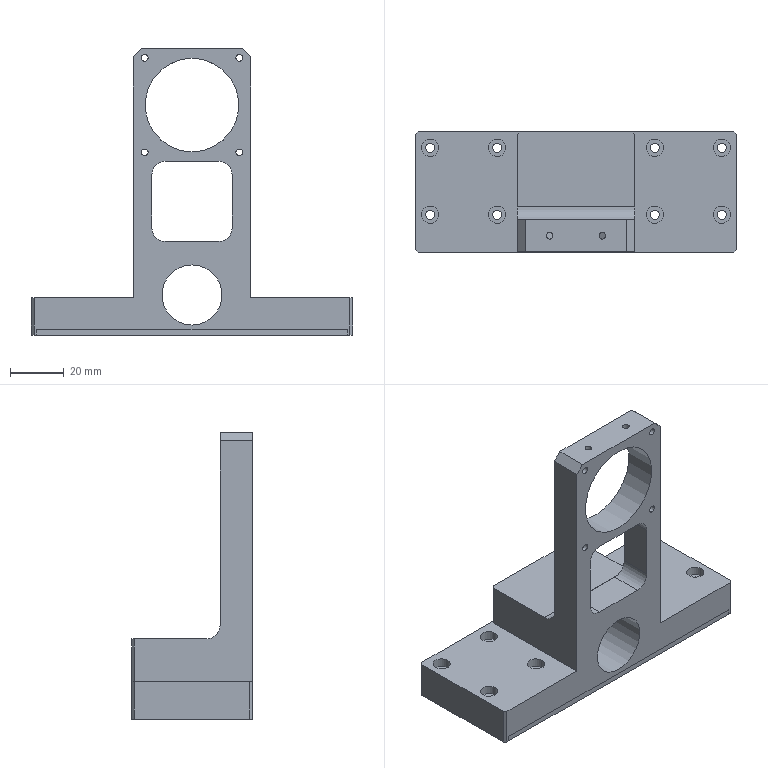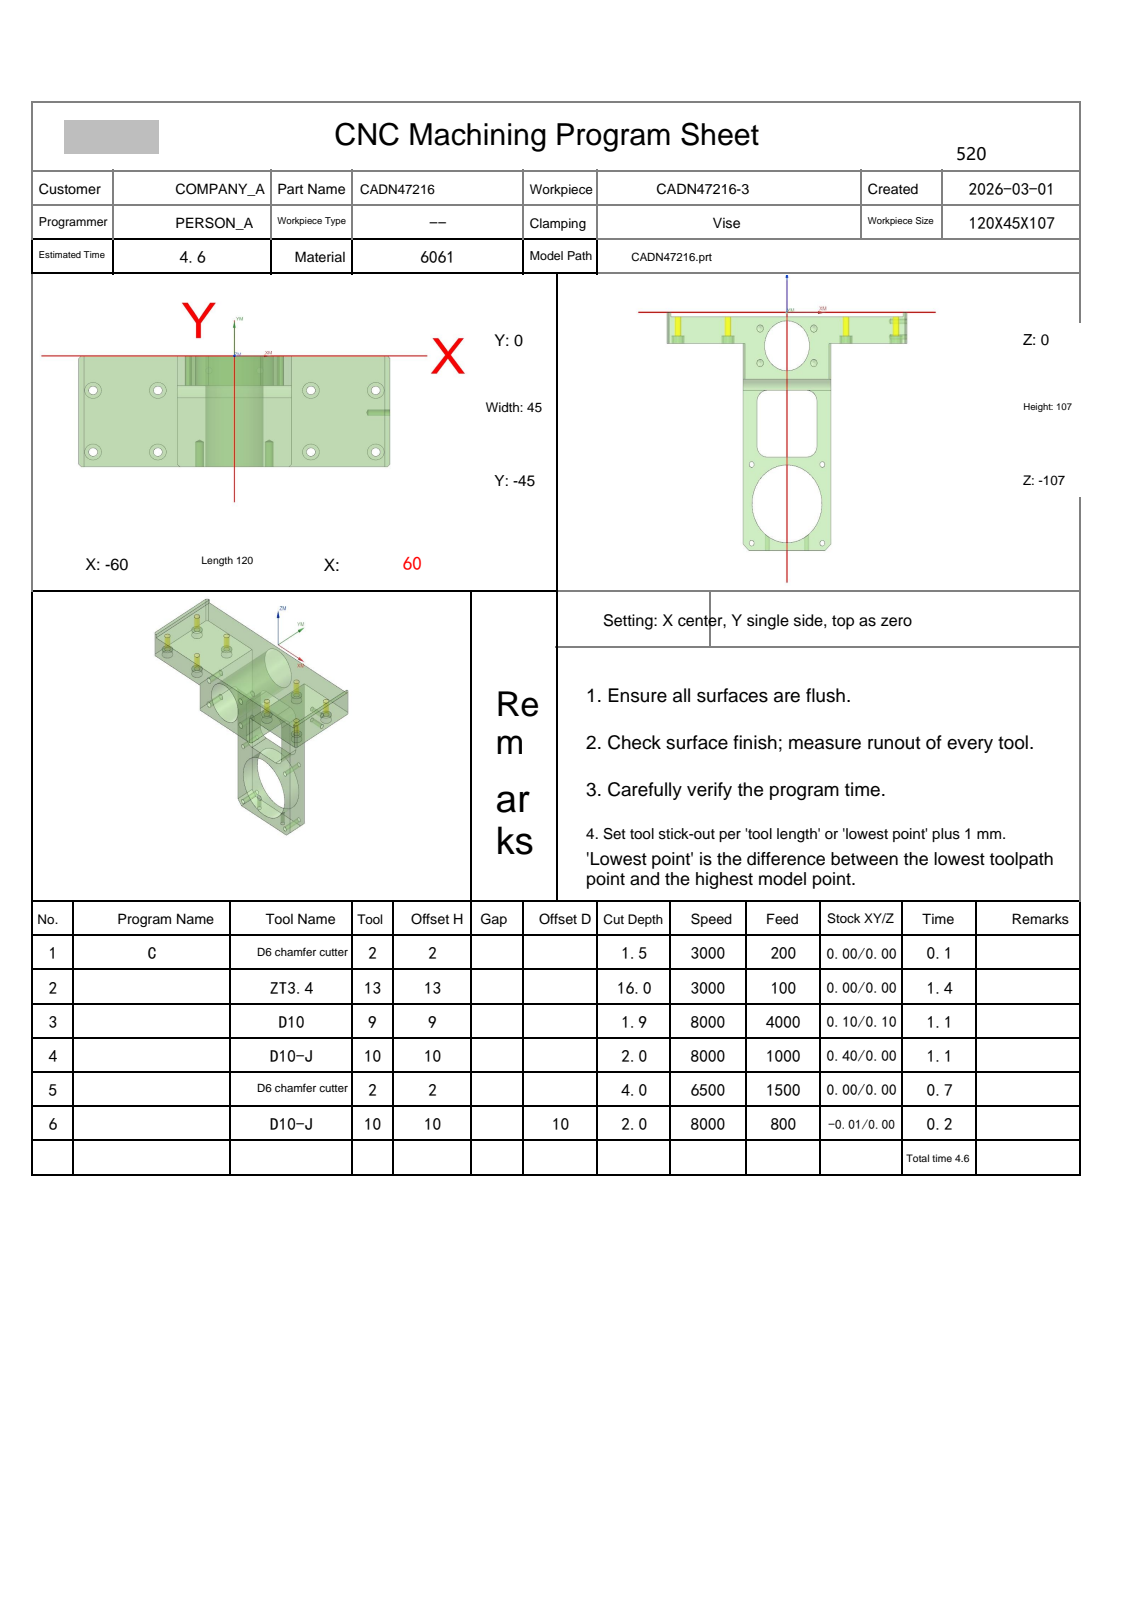NC program | NX | posted by the shop | part box 120 x 45 x 107 mm
Whole program:
%
O0001
(Machine time: 5.76 MIN)
(===Total Tool:4===)
(T2=D6 chamfer cutter   D=6.   R=0.   D-  H02 Z=-4.   )
(T13=ZT3.4  D=3.4  DR_a=118 D-  H13 Z=-16.  )
(T9=D10     D=10.  R=0.   D-  H09 Z=-1.9  )
(T10=D10-J  D=10.  R=0.   D-  H10 Z=-2.   )
G80 G90 G17 G49 G40
G91 G28 Z0
M01
N1 T02 M06
(D6 chamfer cutter  D=6. R=0. H=02 ce=0.00 di=0.00)
G00 G90 G54 X-29.5 Y-14. M03 S3000
G43 H02 Z50.
M08
G98 G81 X-29.5 Y-14. Z-1.5 R1. F200.
X-54.5
Y-39.
X-29.5
X29.5
X54.5
Y-14.
X29.5
G80
G00 Z50.
G91 G28 Z0.0
M05
M09
G91 G28 Z0.0
M01
N2 T13 M06
(ZT3.4 D=3.4 DR_a=118 H=13)
G00 G90 G54 X-29.5 Y-14. M03 S3000
G43 H13 Z50.
M08
G98 G83 X-29.5 Y-14. Z-16. R1. F100. Q1.5
X-54.5
Y-39.
X-29.5
X29.5
X54.5
Y-14.
X29.5
G80
G00 Z50.
G91 G28 Z0.0
M05
M09
G91 G28 Z0.0
M01
N3 T09 M06
(D10  D=10. R=0. H=09 ce=0.10 di=0.10)
G00 G90 G54 X0.0 Y-53. M03 S8000
G43 H09 Z10.1
M08
Z1.025
G01 Z-.475 F4000.
Y-49.9
X-52.9
Y4.9
X52.9
Y-49.9
X3.035
G02 X2.203 Y-49.455 I.001 J1.
G01 X-2.203 Y-42.845
G03 X-3.035 Y-42.4 I-.832 J-.555
G01 X-44.403
G02 X-45.4 Y-41.403 I.003 J1.
G01 Y-3.597
G02 X-44.403 Y-2.6 I1. J-.003
G01 X44.403
G02 X45.4 Y-3.597 I-.003 J-1.
G01 Y-41.403
G02 X44.403 Y-42.4 I-1. J.003
G01 X3.035
G02 X2.203 Y-41.955 I.001 J1.
G01 X-2.203 Y-35.345
G03 X-3.035 Y-34.9 I-.832 J-.555
G01 X-36.903
G02 X-37.9 Y-33.903 I.003 J1.
G01 Y-11.097
G02 X-36.903 Y-10.1 I1. J-.003
G01 X36.903
G02 X37.9 Y-11.097 I-.003 J-1.
G01 Y-33.903
G02 X36.903 Y-34.9 I-1. J.003
G01 X3.035
G02 X2.203 Y-34.455 I0.0 J1.
G01 X-2.203 Y-27.845
G03 X-3.035 Y-27.4 I-.832 J-.555
G01 X-29.403
G02 X-30.4 Y-26.403 I.003 J1.
G01 Y-18.597
G02 X-29.403 Y-17.6 I1. J-.003
G01 X29.403
G02 X30.4 Y-18.597 I-.003 J-1.
G01 Y-26.403
G02 X29.403 Y-27.4 I-1. J.003
G01 X2.664
G02 X1.957 Y-27.107 I0.0 J1.
G01 X-1.957 Y-23.193
G03 X-2.664 Y-22.9 I-.707 J-.707
G01 X-25.502
G02 X-25.9 Y-22.5 I.002 J.4
X-25.502 Y-22.1 I.4 J0.0
G01 X25.502
G02 X25.9 Y-22.5 I-.002 J-.4
X25.502 Y-22.9 I-.4 J0.0
G01 X0.0
X-.5
Y-25.9
Z1.025
G00 X0.0 Y-53.
Z.55
G01 Z-.95
Y-49.9
X-52.9
Y4.9
X52.9
Y-49.9
X3.035
G02 X2.203 Y-49.455 I.001 J1.
G01 X-2.203 Y-42.845
G03 X-3.035 Y-42.4 I-.832 J-.555
G01 X-44.403
G02 X-45.4 Y-41.403 I.003 J1.
G01 Y-3.597
G02 X-44.403 Y-2.6 I1. J-.003
G01 X44.403
G02 X45.4 Y-3.597 I-.003 J-1.
G01 Y-41.403
G02 X44.403 Y-42.4 I-1. J.003
G01 X3.035
G02 X2.203 Y-41.955 I.001 J1.
G01 X-2.203 Y-35.345
G03 X-3.035 Y-34.9 I-.832 J-.555
G01 X-36.903
G02 X-37.9 Y-33.903 I.003 J1.
G01 Y-11.097
G02 X-36.903 Y-10.1 I1. J-.003
G01 X36.903
G02 X37.9 Y-11.097 I-.003 J-1.
G01 Y-33.903
G02 X36.903 Y-34.9 I-1. J.003
G01 X3.035
G02 X2.203 Y-34.455 I0.0 J1.
G01 X-2.203 Y-27.845
G03 X-3.035 Y-27.4 I-.832 J-.555
G01 X-29.403
G02 X-30.4 Y-26.403 I.003 J1.
G01 Y-18.597
G02 X-29.403 Y-17.6 I1. J-.003
G01 X29.403
G02 X30.4 Y-18.597 I-.003 J-1.
G01 Y-26.403
G02 X29.403 Y-27.4 I-1. J.003
G01 X2.664
G02 X1.957 Y-27.107 I0.0 J1.
G01 X-1.957 Y-23.193
G03 X-2.664 Y-22.9 I-.707 J-.707
G01 X-25.502
G02 X-25.9 Y-22.5 I.002 J.4
X-25.502 Y-22.1 I.4 J0.0
G01 X25.502
G02 X25.9 Y-22.5 I-.002 J-.4
X25.502 Y-22.9 I-.4 J0.0
G01 X0.0
X-.5
Y-25.9
Z.55
G00 X0.0 Y-53.
Z.075
G01 Z-1.425
Y-49.9
X-52.9
Y4.9
X52.9
Y-49.9
X3.035
G02 X2.203 Y-49.455 I.001 J1.
G01 X-2.203 Y-42.845
G03 X-3.035 Y-42.4 I-.832 J-.555
G01 X-44.403
G02 X-45.4 Y-41.403 I.003 J1.
G01 Y-3.597
G02 X-44.403 Y-2.6 I1. J-.003
G01 X44.403
G02 X45.4 Y-3.597 I-.003 J-1.
G01 Y-41.403
G02 X44.403 Y-42.4 I-1. J.003
G01 X3.035
G02 X2.203 Y-41.955 I.001 J1.
G01 X-2.203 Y-35.345
G03 X-3.035 Y-34.9 I-.832 J-.555
G01 X-36.903
G02 X-37.9 Y-33.903 I.003 J1.
G01 Y-11.097
G02 X-36.903 Y-10.1 I1. J-.003
G01 X36.903
G02 X37.9 Y-11.097 I-.003 J-1.
G01 Y-33.903
G02 X36.903 Y-34.9 I-1. J.003
G01 X3.035
G02 X2.203 Y-34.455 I0.0 J1.
G01 X-2.203 Y-27.845
G03 X-3.035 Y-27.4 I-.832 J-.555
G01 X-29.403
G02 X-30.4 Y-26.403 I.003 J1.
G01 Y-18.597
G02 X-29.403 Y-17.6 I1. J-.003
G01 X29.403
G02 X30.4 Y-18.597 I-.003 J-1.
G01 Y-26.403
G02 X29.403 Y-27.4 I-1. J.003
G01 X2.664
G02 X1.957 Y-27.107 I0.0 J1.
G01 X-1.957 Y-23.193
G03 X-2.664 Y-22.9 I-.707 J-.707
G01 X-25.502
G02 X-25.9 Y-22.5 I.002 J.4
X-25.502 Y-22.1 I.4 J0.0
G01 X25.502
G02 X25.9 Y-22.5 I-.002 J-.4
X25.502 Y-22.9 I-.4 J0.0
G01 X0.0
X-.5
Y-25.9
Z.075
G00 X0.0 Y-53.
Z-.4
G01 Z-1.9
Y-49.9
X-52.9
Y4.9
X52.9
Y-49.9
X3.035
G02 X2.203 Y-49.455 I.001 J1.
G01 X-2.203 Y-42.845
G03 X-3.035 Y-42.4 I-.832 J-.555
G01 X-44.403
G02 X-45.4 Y-41.403 I.003 J1.
G01 Y-3.597
G02 X-44.403 Y-2.6 I1. J-.003
G01 X44.403
G02 X45.4 Y-3.597 I-.003 J-1.
G01 Y-41.403
G02 X44.403 Y-42.4 I-1. J.003
G01 X3.035
G02 X2.203 Y-41.955 I.001 J1.
G01 X-2.203 Y-35.345
G03 X-3.035 Y-34.9 I-.832 J-.555
G01 X-36.903
G02 X-37.9 Y-33.903 I.003 J1.
G01 Y-11.097
G02 X-36.903 Y-10.1 I1. J-.003
G01 X36.903
G02 X37.9 Y-11.097 I-.003 J-1.
G01 Y-33.903
G02 X36.903 Y-34.9 I-1. J.003
G01 X3.035
G02 X2.203 Y-34.455 I0.0 J1.
G01 X-2.203 Y-27.845
G03 X-3.035 Y-27.4 I-.832 J-.555
G01 X-29.403
G02 X-30.4 Y-26.403 I.003 J1.
G01 Y-18.597
G02 X-29.403 Y-17.6 I1. J-.003
G01 X29.403
G02 X30.4 Y-18.597 I-.003 J-1.
G01 Y-26.403
G02 X29.403 Y-27.4 I-1. J.003
G01 X2.664
G02 X1.957 Y-27.107 I0.0 J1.
G01 X-1.957 Y-23.193
G03 X-2.664 Y-22.9 I-.707 J-.707
G01 X-25.502
G02 X-25.9 Y-22.5 I.002 J.4
X-25.502 Y-22.1 I.4 J0.0
G01 X25.502
G02 X25.9 Y-22.5 I-.002 J-.4
X25.502 Y-22.9 I-.4 J0.0
G01 X0.0
X-.5
Y-25.9
Z-.4
G00 Z10.1
G91 G28 Z0.0
M05
M09
G91 G28 Z0.0
M01
N4 T10 M06
(D10-J  D=10. R=0. H=10 ce=0.40 di=0.00)
G00 G90 G54 X-2. Y7. M03 S8000
G43 H10 Z10.4
M08
Z-.5
G01 Z-2. F1000.
Y3.
G03 X0.0 Y1. I2. J0.0
G01 X51.603
G02 X52.6 Y.003 I-.003 J-1.
G01 Y-45.003
G02 X51.603 Y-46. I-1. J.003
G01 X-51.603
G02 X-52.6 Y-45.003 I.003 J1.
G01 Y.003
G02 X-51.603 Y1. I1. J-.003
G01 X2.086
G02 X2.792 Y.708 I-.001 J-1.
G01 X7.207 Y-3.707
G03 X7.914 Y-4. I.707 J.707
G01 X46.603
G02 X47.6 Y-4.997 I-.003 J-1.
G01 Y-40.003
G02 X46.603 Y-41. I-1. J.003
G01 X-46.603
G02 X-47.6 Y-40.003 I.003 J1.
G01 Y-4.997
G02 X-46.603 Y-4. I1. J-.003
G01 X2.086
G02 X2.792 Y-4.292 I-.001 J-1.
G01 X7.207 Y-8.707
G03 X7.914 Y-9. I.707 J.707
G01 X41.604
G02 X42.6 Y-9.996 I-.004 J-1.
G01 Y-35.004
G02 X41.604 Y-36. I-1. J.004
G01 X-41.604
G02 X-42.6 Y-35.004 I.004 J1.
G01 Y-9.996
G02 X-41.604 Y-9. I1. J-.004
G01 X2.086
G02 X2.793 Y-9.293 I-.001 J-1.
G01 X7.207 Y-13.707
G03 X7.914 Y-14. I.707 J.707
G01 X36.604
G02 X37.6 Y-14.996 I-.004 J-1.
G01 Y-30.004
G02 X36.604 Y-31. I-1. J.004
G01 X-36.604
G02 X-37.6 Y-30.004 I.004 J1.
G01 Y-14.996
G02 X-36.604 Y-14. I1. J-.004
G01 X2.086
G02 X2.793 Y-14.293 I0.0 J-1.
G01 X7.207 Y-18.707
G03 X7.914 Y-19. I.707 J.707
G01 X31.604
G02 X32.6 Y-19.996 I-.004 J-1.
G01 Y-25.004
G02 X31.604 Y-26. I-1. J.004
G01 X-31.604
G02 X-32.6 Y-25.004 I.004 J1.
G01 Y-19.996
G02 X-31.604 Y-19. I1. J-.004
G01 X5.
X6.
G03 X8. Y-17. I0.0 J2.
G01 Z-.5
G00 Z10.4
G91 G28 Z0.0
M05
M09
G91 G28 Z0.0
M01
N5 T02 M06
(D6 chamfer cutter  D=6. R=0. H=02 ce=0.00 di=0.00)
G00 G90 G54 X-29.5 Y-14. M03 S5000
G43 H02 Z50.
M08
G98 G81 X-29.5 Y-14. Z-4. R1. F150.
X-54.5
Y-39.
X-29.5
X29.5
X54.5
Y-14.
X29.5
G80
G00 Z50.
G00 G90 X56.773 Y-22.886 M03 S6500
Z50.
Z.172
G01 Z-1.2 F1500.
G03 X56.973 Y-22.6 I-1.532 J1.286
G01 X57.003 Y-22.554
X57. Y-22.5
Y0.0
G02 X58. Y1. I1. J0.0
G01 X59.
X59.259 Y.966
X59.5 Y.866
X59.707 Y.707
X60.707 Y-.293
X60.866 Y-.5
X60.966 Y-.741
X61. Y-1.
Y-44.
X60.966 Y-44.259
X60.866 Y-44.5
X60.707 Y-44.707
X59.707 Y-45.707
X59.5 Y-45.866
X59.259 Y-45.966
X59. Y-46.
X58.
G02 X57. Y-45. I0.0 J1.
G01 Y-22.5
X57.003 Y-22.446
X56.973 Y-22.4
G03 X56.773 Y-22.114 I-1.732 J-1.
G01 Z.172
G00 Z10.
X-56.773
Z.172
G01 Z-1.2
G03 X-56.973 Y-22.4 I1.532 J-1.286
G01 X-57.003 Y-22.446
X-57. Y-22.5
Y-45.
G02 X-58. Y-46. I-1. J0.0
G01 X-59.
X-59.259 Y-45.966
X-59.5 Y-45.866
X-59.707 Y-45.707
X-60.707 Y-44.707
X-60.866 Y-44.5
X-60.966 Y-44.259
X-61. Y-44.
Y-1.
X-60.966 Y-.741
X-60.866 Y-.5
X-60.707 Y-.293
X-59.707 Y.707
X-59.5 Y.866
X-59.259 Y.966
X-59. Y1.
X-58.
G02 X-57. Y0.0 I0.0 J-1.
G01 Y-22.5
X-57.003 Y-22.554
X-56.973 Y-22.6
G03 X-56.773 Y-22.886 I1.732 J1.
G01 Z.172
G00 Z10.
X-55.029 Y1.068
Z-1.669
G01 Z-3.2
X-54.943 Y1.008
X-54.913 Y1.
X54.913
X54.943 Y1.008
X55.029 Y1.068
Z-1.669
G00 Z10.
Y-46.068
Z-1.669
G01 Z-3.2
X54.943 Y-46.008
X54.913 Y-46.
X-54.913
X-54.943 Y-46.008
X-55.029 Y-46.068
Z-1.669
G00 Z10.
X54.821 Y-13.41
Z-1.623
G01 Z-3.2
X54.774 Y-13.358
X54.756 Y-13.348
G03 X54.5 Y-13.3 I-.256 J-.652
X53.8 Y-14. I0.0 J-.7
X54.5 Y-14.7 I.7 J0.0
X54.756 Y-14.652 I0.0 J.7
G01 X54.774 Y-14.642
X54.821 Y-14.59
Z-1.623
G00 Z10.
Y-38.41
Z-1.623
G01 Z-3.2
X54.774 Y-38.358
X54.756 Y-38.348
G03 X54.5 Y-38.3 I-.256 J-.652
X53.8 Y-39. I0.0 J-.7
X54.5 Y-39.7 I.7 J0.0
X54.756 Y-39.652 I0.0 J.7
G01 X54.774 Y-39.642
X54.821 Y-39.59
Z-1.623
G00 Z10.
X28.974 Y-38.588
Z-1.624
G01 Z-3.2
G03 X28.814 Y-38.897 I1.687 J-1.075
G01 X28.79 Y-38.946
X28.8 Y-39.
G03 X29.5 Y-39.7 I.7 J0.0
X30.2 Y-39. I0.0 J.7
X29.5 Y-38.3 I-.7 J0.0
X28.824 Y-38.819 I0.0 J-.7
G01 X28.8 Y-39.
X28.79 Y-39.054
X28.814 Y-39.103
G03 X28.974 Y-39.412 I1.848 J.765
G01 Z-1.624
G00 Z10.
Y-13.588
Z-1.624
G01 Z-3.2
G03 X28.814 Y-13.897 I1.687 J-1.075
G01 X28.79 Y-13.946
X28.8 Y-14.
G03 X29.5 Y-14.7 I.7 J0.0
X30.2 Y-14. I0.0 J.7
X29.5 Y-13.3 I-.7 J0.0
X28.824 Y-13.819 I0.0 J-.7
G01 X28.8 Y-14.
X28.79 Y-14.054
X28.814 Y-14.103
G03 X28.974 Y-14.412 I1.848 J.765
G01 Z-1.624
G00 Z10.
X-30.026 Y-13.588
Z-1.624
G01 Z-3.2
G03 X-30.186 Y-13.897 I1.687 J-1.075
G01 X-30.21 Y-13.946
X-30.2 Y-14.
G03 X-29.5 Y-14.7 I.7 J0.0
X-28.8 Y-14. I0.0 J.7
X-29.5 Y-13.3 I-.7 J0.0
X-30.176 Y-13.819 I0.0 J-.7
G01 X-30.2 Y-14.
X-30.21 Y-14.054
X-30.186 Y-14.103
G03 X-30.026 Y-14.412 I1.848 J.765
G01 Z-1.624
G00 Z10.
X-54.836 Y-14.539
Z-1.658
G01 Z-3.2
X-54.778 Y-14.626
X-54.753 Y-14.644
X-54.656 Y-14.682
X-54.5 Y-14.7
G03 X-53.8 Y-14. I0.0 J.7
X-54.5 Y-13.3 I-.7 J0.0
G01 X-54.656 Y-13.318
X-54.753 Y-13.356
X-54.778 Y-13.374
X-54.836 Y-13.461
Z-1.658
G00 Z10.
Y-39.539
Z-1.658
G01 Z-3.2
X-54.778 Y-39.626
X-54.753 Y-39.644
X-54.656 Y-39.682
X-54.5 Y-39.7
G03 X-53.8 Y-39. I0.0 J.7
X-54.5 Y-38.3 I-.7 J0.0
G01 X-54.656 Y-38.318
X-54.753 Y-38.356
X-54.778 Y-38.374
X-54.836 Y-38.461
Z-1.658
G00 Z10.
X-30.026 Y-38.588
Z-1.624
G01 Z-3.2
G03 X-30.186 Y-38.897 I1.687 J-1.075
G01 X-30.21 Y-38.946
X-30.2 Y-39.
G03 X-29.5 Y-39.7 I.7 J0.0
X-28.8 Y-39. I0.0 J.7
X-29.5 Y-38.3 I-.7 J0.0
X-30.176 Y-38.819 I0.0 J-.7
G01 X-30.2 Y-39.
X-30.21 Y-39.054
X-30.186 Y-39.103
G03 X-30.026 Y-39.412 I1.848 J.765
G01 Z-1.624
G00 Z50.
G91 G28 Z0.0
M05
M09
G91 G28 Z0.0
M01
N6 T10 M06
(D10-J  D=10. R=0. H=10 ce=-0.01 di=0.00)
G00 G90 G54 X51.061 Y-52.009 M03 S8000
G43 H10 Z10.017
M08
Z-1.
G01 Z-2. F800.
G41 D10
X51.259 Y-51.985
G03 X53.015 Y-50. I-.244 J1.985
G01 Y5.
G03 X51.259 Y6.985 I-2. J0.0
G01 G40 X51.061 Y7.009
Z-1.
G00 X-51.061
G01 Z-2.
G41 D10
X-51.259 Y6.985
G03 X-53.015 Y5. I.244 J-1.985
G01 Y-50.
G03 X-51.259 Y-51.985 I2. J0.0
G01 G40 X-51.061 Y-52.009
Z-1.
G00 Z10.017
M05
M09
G91 G28 Z0.0
G91 G28 Y0.0
M30
%